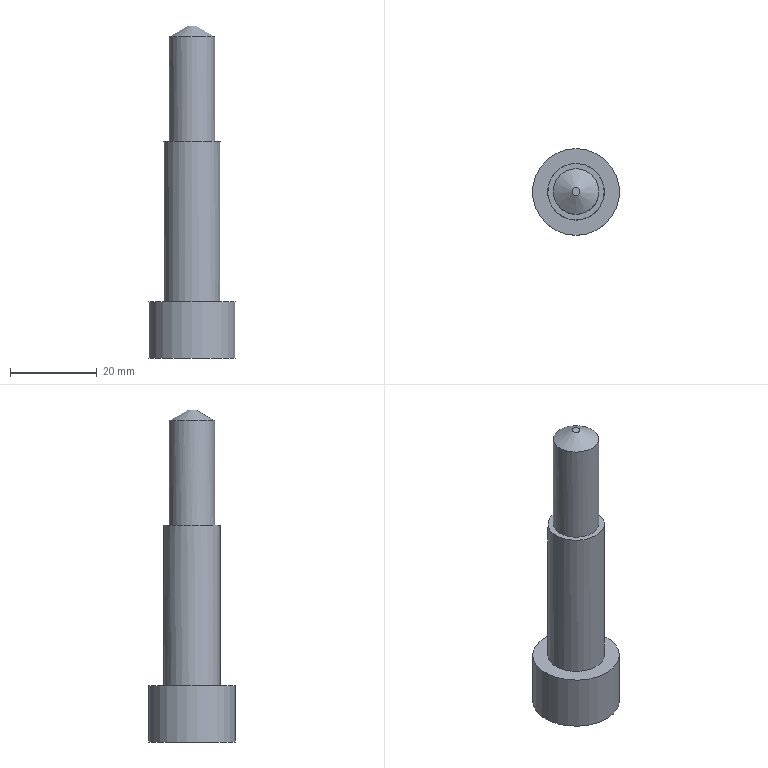Part | STEP file | solid 215 | 1 solid | 8 faces | box 20 x 20 x 76.5 mm | volume 11160 mm3 | plane 4 | cylinder 3 | cone 1 | commonest cylinder face diameters 10.5 x1 13 x1 20 x1